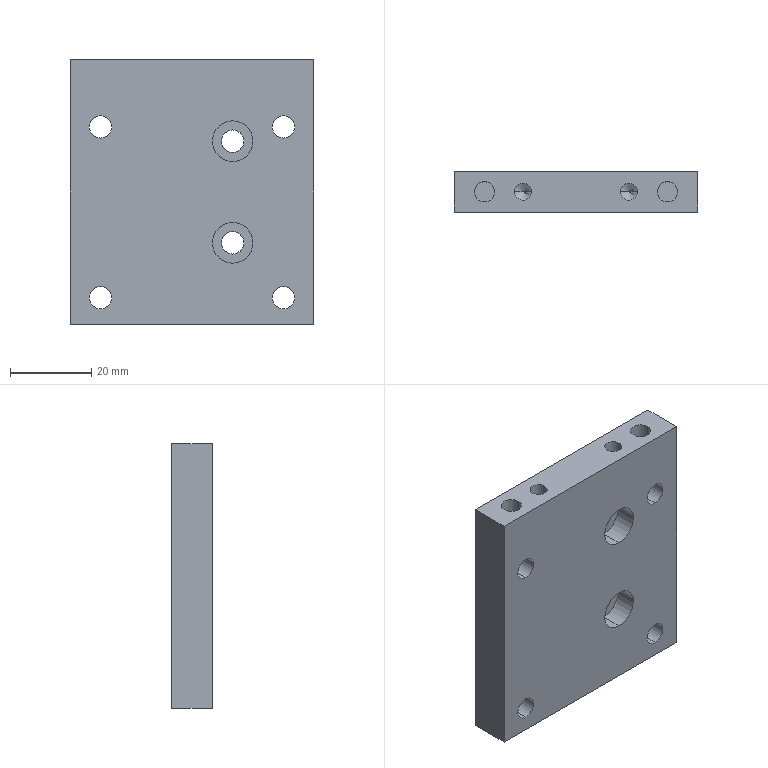Part | SolidWorks | features HoleWzd 4, Extrusion 1 | 1 solid | 50 faces | box 60 x 10 x 65 mm | volume 35169 mm3 | cylinder 32 | plane 14 | cone 4 | commonest cylinder face diameters 5.5 x12 10 x12 4.2 x4 5 x4
STEP:
#1=CARTESIAN_POINT('',(10.,0.4,17.5));
#2=VERTEX_POINT('',#1);
#3=CARTESIAN_POINT('',(10.,0.4,7.5));
#4=VERTEX_POINT('',#3);
#5=CARTESIAN_POINT('',(10.,0.4,12.5));
#6=DIRECTION('',(0.,-1.,0.));
#7=DIRECTION('',(0.,0.,-1.));
#8=AXIS2_PLACEMENT_3D('',#5,#6,#7);
#9=CIRCLE('',#8,5.);
#10=EDGE_CURVE('',#2,#4,#9,.T.);
#11=ORIENTED_EDGE('',*,*,#10,.F.);
#12=CARTESIAN_POINT('',(10.,-5.,17.5));
#13=VERTEX_POINT('',#12);
#14=CARTESIAN_POINT('',(10.,-5.,17.5));
#15=DIRECTION('',(0.,-1.,0.));
#16=VECTOR('',#15,1000.);
#17=LINE('',#14,#16);
#18=EDGE_CURVE('',#2,#13,#17,.T.);
#19=ORIENTED_EDGE('',*,*,#18,.T.);
#20=CARTESIAN_POINT('',(10.,-5.,7.5));
#21=VERTEX_POINT('',#20);
#22=CARTESIAN_POINT('',(10.,-5.,12.5));
#23=DIRECTION('',(0.,-1.,0.));
#24=DIRECTION('',(0.,0.,-1.));
#25=AXIS2_PLACEMENT_3D('',#22,#23,#24);
#26=CIRCLE('',#25,5.);
#27=EDGE_CURVE('',#13,#21,#26,.T.);
#28=ORIENTED_EDGE('',*,*,#27,.T.);
#29=CARTESIAN_POINT('',(10.,-5.,7.5));
#30=DIRECTION('',(0.,-1.,0.));
#31=VECTOR('',#30,1000.);
#32=LINE('',#29,#31);
#33=EDGE_CURVE('',#4,#21,#32,.T.);
#34=ORIENTED_EDGE('',*,*,#33,.F.);
#35=EDGE_LOOP('',(#11,#19,#28,#34));
#36=FACE_OUTER_BOUND('',#35,.T.);
#37=CARTESIAN_POINT('',(10.,-5.,12.5));
#38=DIRECTION('',(0.,-1.,0.));
#39=DIRECTION('',(0.,0.,-1.));
#40=AXIS2_PLACEMENT_3D('',#37,#38,#39);
#41=CYLINDRICAL_SURFACE('',#40,5.);
#42=ADVANCED_FACE('',(#36),#41,.F.);
#43=CARTESIAN_POINT('',(10.,5.,15.25));
#44=VERTEX_POINT('',#43);
#45=CARTESIAN_POINT('',(10.,5.,9.75));
#46=VERTEX_POINT('',#45);
#47=CARTESIAN_POINT('',(10.,5.,12.5));
#48=DIRECTION('',(0.,-1.,0.));
#49=DIRECTION('',(0.,0.,-1.));
#50=AXIS2_PLACEMENT_3D('',#47,#48,#49);
#51=CIRCLE('',#50,2.75);
#52=EDGE_CURVE('',#44,#46,#51,.T.);
#53=ORIENTED_EDGE('',*,*,#52,.F.);
#54=CARTESIAN_POINT('',(10.,0.4,15.25));
#55=VERTEX_POINT('',#54);
#56=CARTESIAN_POINT('',(10.,-5.,15.25));
#57=DIRECTION('',(0.,-1.,0.));
#58=VECTOR('',#57,1000.);
#59=LINE('',#56,#58);
#60=EDGE_CURVE('',#44,#55,#59,.T.);
#61=ORIENTED_EDGE('',*,*,#60,.T.);
#62=CARTESIAN_POINT('',(10.,0.4,9.75));
#63=VERTEX_POINT('',#62);
#64=CARTESIAN_POINT('',(10.,0.4,12.5));
#65=DIRECTION('',(0.,-1.,0.));
#66=DIRECTION('',(0.,0.,-1.));
#67=AXIS2_PLACEMENT_3D('',#64,#65,#66);
#68=CIRCLE('',#67,2.75);
#69=EDGE_CURVE('',#55,#63,#68,.T.);
#70=ORIENTED_EDGE('',*,*,#69,.T.);
#71=CARTESIAN_POINT('',(10.,-5.,9.75));
#72=DIRECTION('',(0.,-1.,0.));
#73=VECTOR('',#72,1000.);
#74=LINE('',#71,#73);
#75=EDGE_CURVE('',#46,#63,#74,.T.);
#76=ORIENTED_EDGE('',*,*,#75,.F.);
#77=EDGE_LOOP('',(#53,#61,#70,#76));
#78=FACE_OUTER_BOUND('',#77,.T.);
#79=CARTESIAN_POINT('',(10.,-5.,12.5));
#80=DIRECTION('',(0.,-1.,0.));
#81=DIRECTION('',(0.,0.,-1.));
#82=AXIS2_PLACEMENT_3D('',#79,#80,#81);
#83=CYLINDRICAL_SURFACE('',#82,2.75);
#84=ADVANCED_FACE('',(#78),#83,.F.);
#85=CARTESIAN_POINT('',(10.,0.4,-7.5));
#86=VERTEX_POINT('',#85);
#87=CARTESIAN_POINT('',(10.,0.4,-17.5));
#88=VERTEX_POINT('',#87);
#89=CARTESIAN_POINT('',(10.,0.4,-12.5));
#90=DIRECTION('',(0.,-1.,0.));
#91=DIRECTION('',(0.,0.,-1.));
#92=AXIS2_PLACEMENT_3D('',#89,#90,#91);
#93=CIRCLE('',#92,5.);
#94=EDGE_CURVE('',#86,#88,#93,.T.);
#95=ORIENTED_EDGE('',*,*,#94,.F.);
#96=CARTESIAN_POINT('',(10.,-5.,-7.5));
#97=VERTEX_POINT('',#96);
#98=CARTESIAN_POINT('',(10.,-5.,-7.5));
#99=DIRECTION('',(0.,-1.,0.));
#100=VECTOR('',#99,1000.);
#101=LINE('',#98,#100);
#102=EDGE_CURVE('',#86,#97,#101,.T.);
#103=ORIENTED_EDGE('',*,*,#102,.T.);
#104=CARTESIAN_POINT('',(10.,-5.,-17.5));
#105=VERTEX_POINT('',#104);
#106=CARTESIAN_POINT('',(10.,-5.,-12.5));
#107=DIRECTION('',(0.,-1.,0.));
#108=DIRECTION('',(0.,0.,-1.));
#109=AXIS2_PLACEMENT_3D('',#106,#107,#108);
#110=CIRCLE('',#109,5.);
#111=EDGE_CURVE('',#97,#105,#110,.T.);
#112=ORIENTED_EDGE('',*,*,#111,.T.);
#113=CARTESIAN_POINT('',(10.,-5.,-17.5));
#114=DIRECTION('',(0.,-1.,0.));
#115=VECTOR('',#114,1000.);
#116=LINE('',#113,#115);
#117=EDGE_CURVE('',#88,#105,#116,.T.);
#118=ORIENTED_EDGE('',*,*,#117,.F.);
#119=EDGE_LOOP('',(#95,#103,#112,#118));
#120=FACE_OUTER_BOUND('',#119,.T.);
#121=CARTESIAN_POINT('',(10.,-5.,-12.5));
#122=DIRECTION('',(0.,-1.,0.));
#123=DIRECTION('',(0.,0.,-1.));
#124=AXIS2_PLACEMENT_3D('',#121,#122,#123);
#125=CYLINDRICAL_SURFACE('',#124,5.);
#126=ADVANCED_FACE('',(#120),#125,.F.);
#127=CARTESIAN_POINT('',(10.,5.,-9.75));
#128=VERTEX_POINT('',#127);
#129=CARTESIAN_POINT('',(10.,5.,-15.25));
#130=VERTEX_POINT('',#129);
#131=CARTESIAN_POINT('',(10.,5.,-12.5));
#132=DIRECTION('',(0.,-1.,0.));
#133=DIRECTION('',(0.,0.,-1.));
#134=AXIS2_PLACEMENT_3D('',#131,#132,#133);
#135=CIRCLE('',#134,2.75);
#136=EDGE_CURVE('',#128,#130,#135,.T.);
#137=ORIENTED_EDGE('',*,*,#136,.F.);
#138=CARTESIAN_POINT('',(10.,0.4,-9.75));
#139=VERTEX_POINT('',#138);
#140=CARTESIAN_POINT('',(10.,-5.,-9.75));
#141=DIRECTION('',(0.,-1.,0.));
#142=VECTOR('',#141,1000.);
#143=LINE('',#140,#142);
#144=EDGE_CURVE('',#128,#139,#143,.T.);
#145=ORIENTED_EDGE('',*,*,#144,.T.);
#146=CARTESIAN_POINT('',(10.,0.4,-15.25));
#147=VERTEX_POINT('',#146);
#148=CARTESIAN_POINT('',(10.,0.4,-12.5));
#149=DIRECTION('',(0.,-1.,0.));
#150=DIRECTION('',(0.,0.,-1.));
#151=AXIS2_PLACEMENT_3D('',#148,#149,#150);
#152=CIRCLE('',#151,2.75);
#153=EDGE_CURVE('',#139,#147,#152,.T.);
#154=ORIENTED_EDGE('',*,*,#153,.T.);
#155=CARTESIAN_POINT('',(10.,-5.,-15.25));
#156=DIRECTION('',(0.,-1.,0.));
#157=VECTOR('',#156,1000.);
#158=LINE('',#155,#157);
#159=EDGE_CURVE('',#130,#147,#158,.T.);
#160=ORIENTED_EDGE('',*,*,#159,.F.);
#161=EDGE_LOOP('',(#137,#145,#154,#160));
#162=FACE_OUTER_BOUND('',#161,.T.);
#163=CARTESIAN_POINT('',(10.,-5.,-12.5));
#164=DIRECTION('',(0.,-1.,0.));
#165=DIRECTION('',(0.,0.,-1.));
#166=AXIS2_PLACEMENT_3D('',#163,#164,#165);
#167=CYLINDRICAL_SURFACE('',#166,2.75);
#168=ADVANCED_FACE('',(#162),#167,.F.);
#169=CARTESIAN_POINT('',(-15.1,0.,20.1));
#170=VERTEX_POINT('',#169);
#171=CARTESIAN_POINT('',(-10.9,0.,20.1));
#172=VERTEX_POINT('',#171);
#173=CARTESIAN_POINT('',(-13.,0.,20.1));
#174=DIRECTION('',(0.,0.,1.));
#175=DIRECTION('',(1.,0.,0.));
#176=AXIS2_PLACEMENT_3D('',#173,#174,#175);
#177=CIRCLE('',#176,2.1);
#178=EDGE_CURVE('',#170,#172,#177,.T.);
#179=ORIENTED_EDGE('',*,*,#178,.F.);
#180=CARTESIAN_POINT('',(-15.1,0.,32.5));
#181=VERTEX_POINT('',#180);
#182=CARTESIAN_POINT('',(-15.1,0.,32.5));
#183=DIRECTION('',(0.,0.,1.));
#184=VECTOR('',#183,1000.);
#185=LINE('',#182,#184);
#186=EDGE_CURVE('',#170,#181,#185,.T.);
#187=ORIENTED_EDGE('',*,*,#186,.T.);
#188=CARTESIAN_POINT('',(-10.9,0.,32.5));
#189=VERTEX_POINT('',#188);
#190=CARTESIAN_POINT('',(-13.,0.,32.5));
#191=DIRECTION('',(0.,0.,1.));
#192=DIRECTION('',(1.,0.,0.));
#193=AXIS2_PLACEMENT_3D('',#190,#191,#192);
#194=CIRCLE('',#193,2.1);
#195=EDGE_CURVE('',#181,#189,#194,.T.);
#196=ORIENTED_EDGE('',*,*,#195,.T.);
#197=CARTESIAN_POINT('',(-10.9,0.,32.5));
#198=DIRECTION('',(0.,0.,1.));
#199=VECTOR('',#198,1000.);
#200=LINE('',#197,#199);
#201=EDGE_CURVE('',#172,#189,#200,.T.);
#202=ORIENTED_EDGE('',*,*,#201,.F.);
#203=EDGE_LOOP('',(#179,#187,#196,#202));
#204=FACE_OUTER_BOUND('',#203,.T.);
#205=CARTESIAN_POINT('',(-13.,0.,32.5));
#206=DIRECTION('',(0.,0.,1.));
#207=DIRECTION('',(1.,0.,0.));
#208=AXIS2_PLACEMENT_3D('',#205,#206,#207);
#209=CYLINDRICAL_SURFACE('',#208,2.1);
#210=ADVANCED_FACE('',(#204),#209,.F.);
#211=CARTESIAN_POINT('',(-13.,0.,18.838));
#212=VERTEX_POINT('',#211);
#213=CARTESIAN_POINT('',(-10.9,0.,20.1));
#214=DIRECTION('',(0.8572,0.,0.515));
#215=VECTOR('',#214,1000.);
#216=LINE('',#213,#215);
#217=EDGE_CURVE('',#212,#172,#216,.T.);
#218=ORIENTED_EDGE('',*,*,#217,.F.);
#219=CARTESIAN_POINT('',(-15.1,0.,20.1));
#220=DIRECTION('',(-0.8572,0.,0.515));
#221=VECTOR('',#220,1000.);
#222=LINE('',#219,#221);
#223=EDGE_CURVE('',#212,#170,#222,.T.);
#224=ORIENTED_EDGE('',*,*,#223,.T.);
#225=ORIENTED_EDGE('',*,*,#178,.T.);
#226=EDGE_LOOP('',(#218,#224,#225));
#227=FACE_OUTER_BOUND('',#226,.T.);
#228=CARTESIAN_POINT('',(-13.,0.,20.1));
#229=DIRECTION('',(0.,0.,1.));
#230=DIRECTION('',(1.,0.,0.));
#231=AXIS2_PLACEMENT_3D('',#228,#229,#230);
#232=CONICAL_SURFACE('',#231,2.1,1.03);
#233=ADVANCED_FACE('',(#227),#232,.F.);
#234=CARTESIAN_POINT('',(10.9,0.,20.1));
#235=VERTEX_POINT('',#234);
#236=CARTESIAN_POINT('',(15.1,0.,20.1));
#237=VERTEX_POINT('',#236);
#238=CARTESIAN_POINT('',(13.,0.,20.1));
#239=DIRECTION('',(0.,0.,1.));
#240=DIRECTION('',(1.,0.,0.));
#241=AXIS2_PLACEMENT_3D('',#238,#239,#240);
#242=CIRCLE('',#241,2.1);
#243=EDGE_CURVE('',#235,#237,#242,.T.);
#244=ORIENTED_EDGE('',*,*,#243,.F.);
#245=CARTESIAN_POINT('',(10.9,0.,32.5));
#246=VERTEX_POINT('',#245);
#247=CARTESIAN_POINT('',(10.9,0.,32.5));
#248=DIRECTION('',(0.,0.,1.));
#249=VECTOR('',#248,1000.);
#250=LINE('',#247,#249);
#251=EDGE_CURVE('',#235,#246,#250,.T.);
#252=ORIENTED_EDGE('',*,*,#251,.T.);
#253=CARTESIAN_POINT('',(15.1,0.,32.5));
#254=VERTEX_POINT('',#253);
#255=CARTESIAN_POINT('',(13.,0.,32.5));
#256=DIRECTION('',(0.,0.,1.));
#257=DIRECTION('',(1.,0.,0.));
#258=AXIS2_PLACEMENT_3D('',#255,#256,#257);
#259=CIRCLE('',#258,2.1);
#260=EDGE_CURVE('',#246,#254,#259,.T.);
#261=ORIENTED_EDGE('',*,*,#260,.T.);
#262=CARTESIAN_POINT('',(15.1,0.,32.5));
#263=DIRECTION('',(0.,0.,1.));
#264=VECTOR('',#263,1000.);
#265=LINE('',#262,#264);
#266=EDGE_CURVE('',#237,#254,#265,.T.);
#267=ORIENTED_EDGE('',*,*,#266,.F.);
#268=EDGE_LOOP('',(#244,#252,#261,#267));
#269=FACE_OUTER_BOUND('',#268,.T.);
#270=CARTESIAN_POINT('',(13.,0.,32.5));
#271=DIRECTION('',(0.,0.,1.));
#272=DIRECTION('',(1.,0.,0.));
#273=AXIS2_PLACEMENT_3D('',#270,#271,#272);
#274=CYLINDRICAL_SURFACE('',#273,2.1);
#275=ADVANCED_FACE('',(#269),#274,.F.);
#276=CARTESIAN_POINT('',(13.,0.,18.838));
#277=VERTEX_POINT('',#276);
#278=CARTESIAN_POINT('',(15.1,0.,20.1));
#279=DIRECTION('',(0.8572,0.,0.515));
#280=VECTOR('',#279,1000.);
#281=LINE('',#278,#280);
#282=EDGE_CURVE('',#277,#237,#281,.T.);
#283=ORIENTED_EDGE('',*,*,#282,.F.);
#284=CARTESIAN_POINT('',(10.9,0.,20.1));
#285=DIRECTION('',(-0.8572,0.,0.515));
#286=VECTOR('',#285,1000.);
#287=LINE('',#284,#286);
#288=EDGE_CURVE('',#277,#235,#287,.T.);
#289=ORIENTED_EDGE('',*,*,#288,.T.);
#290=ORIENTED_EDGE('',*,*,#243,.T.);
#291=EDGE_LOOP('',(#283,#289,#290));
#292=FACE_OUTER_BOUND('',#291,.T.);
#293=CARTESIAN_POINT('',(13.,0.,20.1));
#294=DIRECTION('',(0.,0.,1.));
#295=DIRECTION('',(1.,0.,0.));
#296=AXIS2_PLACEMENT_3D('',#293,#294,#295);
#297=CONICAL_SURFACE('',#296,2.1,1.03);
#298=ADVANCED_FACE('',(#292),#297,.F.);
#299=CARTESIAN_POINT('',(-25.,0.,25.5));
#300=VERTEX_POINT('',#299);
#301=CARTESIAN_POINT('',(-20.,0.,25.5));
#302=VERTEX_POINT('',#301);
#303=CARTESIAN_POINT('',(-22.5,0.,25.5));
#304=DIRECTION('',(0.,0.,1.));
#305=DIRECTION('',(1.,0.,0.));
#306=AXIS2_PLACEMENT_3D('',#303,#304,#305);
#307=CIRCLE('',#306,2.5);
#308=EDGE_CURVE('',#300,#302,#307,.T.);
#309=ORIENTED_EDGE('',*,*,#308,.F.);
#310=CARTESIAN_POINT('',(-25.,0.,32.5));
#311=VERTEX_POINT('',#310);
#312=CARTESIAN_POINT('',(-25.,0.,32.5));
#313=DIRECTION('',(0.,0.,1.));
#314=VECTOR('',#313,1000.);
#315=LINE('',#312,#314);
#316=EDGE_CURVE('',#300,#311,#315,.T.);
#317=ORIENTED_EDGE('',*,*,#316,.T.);
#318=CARTESIAN_POINT('',(-20.,0.,32.5));
#319=VERTEX_POINT('',#318);
#320=CARTESIAN_POINT('',(-22.5,0.,32.5));
#321=DIRECTION('',(0.,0.,1.));
#322=DIRECTION('',(1.,0.,0.));
#323=AXIS2_PLACEMENT_3D('',#320,#321,#322);
#324=CIRCLE('',#323,2.5);
#325=EDGE_CURVE('',#311,#319,#324,.T.);
#326=ORIENTED_EDGE('',*,*,#325,.T.);
#327=CARTESIAN_POINT('',(-20.,0.,32.5));
#328=DIRECTION('',(0.,0.,1.));
#329=VECTOR('',#328,1000.);
#330=LINE('',#327,#329);
#331=EDGE_CURVE('',#302,#319,#330,.T.);
#332=ORIENTED_EDGE('',*,*,#331,.F.);
#333=EDGE_LOOP('',(#309,#317,#326,#332));
#334=FACE_OUTER_BOUND('',#333,.T.);
#335=CARTESIAN_POINT('',(-22.5,0.,32.5));
#336=DIRECTION('',(0.,0.,1.));
#337=DIRECTION('',(1.,0.,0.));
#338=AXIS2_PLACEMENT_3D('',#335,#336,#337);
#339=CYLINDRICAL_SURFACE('',#338,2.5);
#340=ADVANCED_FACE('',(#334),#339,.F.);
#341=CARTESIAN_POINT('',(20.,0.,25.5));
#342=VERTEX_POINT('',#341);
#343=CARTESIAN_POINT('',(25.,0.,25.5));
#344=VERTEX_POINT('',#343);
#345=CARTESIAN_POINT('',(22.5,0.,25.5));
#346=DIRECTION('',(0.,0.,1.));
#347=DIRECTION('',(1.,0.,0.));
#348=AXIS2_PLACEMENT_3D('',#345,#346,#347);
#349=CIRCLE('',#348,2.5);
#350=EDGE_CURVE('',#342,#344,#349,.T.);
#351=ORIENTED_EDGE('',*,*,#350,.F.);
#352=CARTESIAN_POINT('',(20.,0.,32.5));
#353=VERTEX_POINT('',#352);
#354=CARTESIAN_POINT('',(20.,0.,32.5));
#355=DIRECTION('',(0.,0.,1.));
#356=VECTOR('',#355,1000.);
#357=LINE('',#354,#356);
#358=EDGE_CURVE('',#342,#353,#357,.T.);
#359=ORIENTED_EDGE('',*,*,#358,.T.);
#360=CARTESIAN_POINT('',(25.,0.,32.5));
#361=VERTEX_POINT('',#360);
#362=CARTESIAN_POINT('',(22.5,0.,32.5));
#363=DIRECTION('',(0.,0.,1.));
#364=DIRECTION('',(1.,0.,0.));
#365=AXIS2_PLACEMENT_3D('',#362,#363,#364);
#366=CIRCLE('',#365,2.5);
#367=EDGE_CURVE('',#353,#361,#366,.T.);
#368=ORIENTED_EDGE('',*,*,#367,.T.);
#369=CARTESIAN_POINT('',(25.,0.,32.5));
#370=DIRECTION('',(0.,0.,1.));
#371=VECTOR('',#370,1000.);
#372=LINE('',#369,#371);
#373=EDGE_CURVE('',#344,#361,#372,.T.);
#374=ORIENTED_EDGE('',*,*,#373,.F.);
#375=EDGE_LOOP('',(#351,#359,#368,#374));
#376=FACE_OUTER_BOUND('',#375,.T.);
#377=CARTESIAN_POINT('',(22.5,0.,32.5));
#378=DIRECTION('',(0.,0.,1.));
#379=DIRECTION('',(1.,0.,0.));
#380=AXIS2_PLACEMENT_3D('',#377,#378,#379);
#381=CYLINDRICAL_SURFACE('',#380,2.5);
#382=ADVANCED_FACE('',(#376),#381,.F.);
#383=CARTESIAN_POINT('',(-22.5,-0.4,-31.));
#384=VERTEX_POINT('',#383);
#385=CARTESIAN_POINT('',(-22.5,-0.4,-21.));
#386=VERTEX_POINT('',#385);
#387=CARTESIAN_POINT('',(-22.5,-0.4,-26.));
#388=DIRECTION('',(0.,1.,0.));
#389=DIRECTION('',(0.,0.,1.));
#390=AXIS2_PLACEMENT_3D('',#387,#388,#389);
#391=CIRCLE('',#390,5.);
#392=EDGE_CURVE('',#384,#386,#391,.T.);
#393=ORIENTED_EDGE('',*,*,#392,.F.);
#394=CARTESIAN_POINT('',(-22.5,5.,-31.));
#395=VERTEX_POINT('',#394);
#396=CARTESIAN_POINT('',(-22.5,5.,-31.));
#397=DIRECTION('',(0.,1.,0.));
#398=VECTOR('',#397,1000.);
#399=LINE('',#396,#398);
#400=EDGE_CURVE('',#384,#395,#399,.T.);
#401=ORIENTED_EDGE('',*,*,#400,.T.);
#402=CARTESIAN_POINT('',(-22.5,5.,-21.));
#403=VERTEX_POINT('',#402);
#404=CARTESIAN_POINT('',(-22.5,5.,-26.));
#405=DIRECTION('',(0.,1.,0.));
#406=DIRECTION('',(0.,0.,1.));
#407=AXIS2_PLACEMENT_3D('',#404,#405,#406);
#408=CIRCLE('',#407,5.);
#409=EDGE_CURVE('',#395,#403,#408,.T.);
#410=ORIENTED_EDGE('',*,*,#409,.T.);
#411=CARTESIAN_POINT('',(-22.5,5.,-21.));
#412=DIRECTION('',(0.,1.,0.));
#413=VECTOR('',#412,1000.);
#414=LINE('',#411,#413);
#415=EDGE_CURVE('',#386,#403,#414,.T.);
#416=ORIENTED_EDGE('',*,*,#415,.F.);
#417=EDGE_LOOP('',(#393,#401,#410,#416));
#418=FACE_OUTER_BOUND('',#417,.T.);
#419=CARTESIAN_POINT('',(-22.5,5.,-26.));
#420=DIRECTION('',(0.,1.,0.));
#421=DIRECTION('',(0.,0.,1.));
#422=AXIS2_PLACEMENT_3D('',#419,#420,#421);
#423=CYLINDRICAL_SURFACE('',#422,5.);
#424=ADVANCED_FACE('',(#418),#423,.F.);
#425=CARTESIAN_POINT('',(-22.5,-5.,-28.75));
#426=VERTEX_POINT('',#425);
#427=CARTESIAN_POINT('',(-22.5,-5.,-23.25));
#428=VERTEX_POINT('',#427);
#429=CARTESIAN_POINT('',(-22.5,-5.,-26.));
#430=DIRECTION('',(0.,1.,0.));
#431=DIRECTION('',(0.,0.,1.));
#432=AXIS2_PLACEMENT_3D('',#429,#430,#431);
#433=CIRCLE('',#432,2.75);
#434=EDGE_CURVE('',#426,#428,#433,.T.);
#435=ORIENTED_EDGE('',*,*,#434,.F.);
#436=CARTESIAN_POINT('',(-22.5,-0.4,-28.75));
#437=VERTEX_POINT('',#436);
#438=CARTESIAN_POINT('',(-22.5,5.,-28.75));
#439=DIRECTION('',(0.,1.,0.));
#440=VECTOR('',#439,1000.);
#441=LINE('',#438,#440);
#442=EDGE_CURVE('',#426,#437,#441,.T.);
#443=ORIENTED_EDGE('',*,*,#442,.T.);
#444=CARTESIAN_POINT('',(-22.5,-0.4,-23.25));
#445=VERTEX_POINT('',#444);
#446=CARTESIAN_POINT('',(-22.5,-0.4,-26.));
#447=DIRECTION('',(0.,1.,0.));
#448=DIRECTION('',(0.,0.,1.));
#449=AXIS2_PLACEMENT_3D('',#446,#447,#448);
#450=CIRCLE('',#449,2.75);
#451=EDGE_CURVE('',#437,#445,#450,.T.);
#452=ORIENTED_EDGE('',*,*,#451,.T.);
#453=CARTESIAN_POINT('',(-22.5,5.,-23.25));
#454=DIRECTION('',(0.,1.,0.));
#455=VECTOR('',#454,1000.);
#456=LINE('',#453,#455);
#457=EDGE_CURVE('',#428,#445,#456,.T.);
#458=ORIENTED_EDGE('',*,*,#457,.F.);
#459=EDGE_LOOP('',(#435,#443,#452,#458));
#460=FACE_OUTER_BOUND('',#459,.T.);
#461=CARTESIAN_POINT('',(-22.5,5.,-26.));
#462=DIRECTION('',(0.,1.,0.));
#463=DIRECTION('',(0.,0.,1.));
#464=AXIS2_PLACEMENT_3D('',#461,#462,#463);
#465=CYLINDRICAL_SURFACE('',#464,2.75);
#466=ADVANCED_FACE('',(#460),#465,.F.);
#467=CARTESIAN_POINT('',(-22.5,-0.4,11.));
#468=VERTEX_POINT('',#467);
#469=CARTESIAN_POINT('',(-22.5,-0.4,21.));
#470=VERTEX_POINT('',#469);
#471=CARTESIAN_POINT('',(-22.5,-0.4,16.));
#472=DIRECTION('',(0.,1.,0.));
#473=DIRECTION('',(0.,0.,1.));
#474=AXIS2_PLACEMENT_3D('',#471,#472,#473);
#475=CIRCLE('',#474,5.);
#476=EDGE_CURVE('',#468,#470,#475,.T.);
#477=ORIENTED_EDGE('',*,*,#476,.F.);
#478=CARTESIAN_POINT('',(-22.5,5.,11.));
#479=VERTEX_POINT('',#478);
#480=CARTESIAN_POINT('',(-22.5,5.,11.));
#481=DIRECTION('',(0.,1.,0.));
#482=VECTOR('',#481,1000.);
#483=LINE('',#480,#482);
#484=EDGE_CURVE('',#468,#479,#483,.T.);
#485=ORIENTED_EDGE('',*,*,#484,.T.);
#486=CARTESIAN_POINT('',(-22.5,5.,21.));
#487=VERTEX_POINT('',#486);
#488=CARTESIAN_POINT('',(-22.5,5.,16.));
#489=DIRECTION('',(0.,1.,0.));
#490=DIRECTION('',(0.,0.,1.));
#491=AXIS2_PLACEMENT_3D('',#488,#489,#490);
#492=CIRCLE('',#491,5.);
#493=EDGE_CURVE('',#479,#487,#492,.T.);
#494=ORIENTED_EDGE('',*,*,#493,.T.);
#495=CARTESIAN_POINT('',(-22.5,5.,21.));
#496=DIRECTION('',(0.,1.,0.));
#497=VECTOR('',#496,1000.);
#498=LINE('',#495,#497);
#499=EDGE_CURVE('',#470,#487,#498,.T.);
#500=ORIENTED_EDGE('',*,*,#499,.F.);
#501=EDGE_LOOP('',(#477,#485,#494,#500));
#502=FACE_OUTER_BOUND('',#501,.T.);
#503=CARTESIAN_POINT('',(-22.5,5.,16.));
#504=DIRECTION('',(0.,1.,0.));
#505=DIRECTION('',(0.,0.,1.));
#506=AXIS2_PLACEMENT_3D('',#503,#504,#505);
#507=CYLINDRICAL_SURFACE('',#506,5.);
#508=ADVANCED_FACE('',(#502),#507,.F.);
#509=CARTESIAN_POINT('',(-22.5,-5.,13.25));
#510=VERTEX_POINT('',#509);
#511=CARTESIAN_POINT('',(-22.5,-5.,18.75));
#512=VERTEX_POINT('',#511);
#513=CARTESIAN_POINT('',(-22.5,-5.,16.));
#514=DIRECTION('',(0.,1.,0.));
#515=DIRECTION('',(0.,0.,1.));
#516=AXIS2_PLACEMENT_3D('',#513,#514,#515);
#517=CIRCLE('',#516,2.75);
#518=EDGE_CURVE('',#510,#512,#517,.T.);
#519=ORIENTED_EDGE('',*,*,#518,.F.);
#520=CARTESIAN_POINT('',(-22.5,-0.4,13.25));
#521=VERTEX_POINT('',#520);
#522=CARTESIAN_POINT('',(-22.5,5.,13.25));
#523=DIRECTION('',(0.,1.,0.));
#524=VECTOR('',#523,1000.);
#525=LINE('',#522,#524);
#526=EDGE_CURVE('',#510,#521,#525,.T.);
#527=ORIENTED_EDGE('',*,*,#526,.T.);
#528=CARTESIAN_POINT('',(-22.5,-0.4,18.75));
#529=VERTEX_POINT('',#528);
#530=CARTESIAN_POINT('',(-22.5,-0.4,16.));
#531=DIRECTION('',(0.,1.,0.));
#532=DIRECTION('',(0.,0.,1.));
#533=AXIS2_PLACEMENT_3D('',#530,#531,#532);
#534=CIRCLE('',#533,2.75);
#535=EDGE_CURVE('',#521,#529,#534,.T.);
#536=ORIENTED_EDGE('',*,*,#535,.T.);
#537=CARTESIAN_POINT('',(-22.5,5.,18.75));
#538=DIRECTION('',(0.,1.,0.));
#539=VECTOR('',#538,1000.);
#540=LINE('',#537,#539);
#541=EDGE_CURVE('',#512,#529,#540,.T.);
#542=ORIENTED_EDGE('',*,*,#541,.F.);
#543=EDGE_LOOP('',(#519,#527,#536,#542));
#544=FACE_OUTER_BOUND('',#543,.T.);
#545=CARTESIAN_POINT('',(-22.5,5.,16.));
#546=DIRECTION('',(0.,1.,0.));
#547=DIRECTION('',(0.,0.,1.));
#548=AXIS2_PLACEMENT_3D('',#545,#546,#547);
#549=CYLINDRICAL_SURFACE('',#548,2.75);
#550=ADVANCED_FACE('',(#544),#549,.F.);
#551=CARTESIAN_POINT('',(22.5,-0.4,11.));
#552=VERTEX_POINT('',#551);
#553=CARTESIAN_POINT('',(22.5,-0.4,21.));
#554=VERTEX_POINT('',#553);
#555=CARTESIAN_POINT('',(22.5,-0.4,16.));
#556=DIRECTION('',(0.,1.,0.));
#557=DIRECTION('',(0.,0.,1.));
#558=AXIS2_PLACEMENT_3D('',#555,#556,#557);
#559=CIRCLE('',#558,5.);
#560=EDGE_CURVE('',#552,#554,#559,.T.);
#561=ORIENTED_EDGE('',*,*,#560,.F.);
#562=CARTESIAN_POINT('',(22.5,5.,11.));
#563=VERTEX_POINT('',#562);
#564=CARTESIAN_POINT('',(22.5,5.,11.));
#565=DIRECTION('',(0.,1.,0.));
#566=VECTOR('',#565,1000.);
#567=LINE('',#564,#566);
#568=EDGE_CURVE('',#552,#563,#567,.T.);
#569=ORIENTED_EDGE('',*,*,#568,.T.);
#570=CARTESIAN_POINT('',(22.5,5.,21.));
#571=VERTEX_POINT('',#570);
#572=CARTESIAN_POINT('',(22.5,5.,16.));
#573=DIRECTION('',(0.,1.,0.));
#574=DIRECTION('',(0.,0.,1.));
#575=AXIS2_PLACEMENT_3D('',#572,#573,#574);
#576=CIRCLE('',#575,5.);
#577=EDGE_CURVE('',#563,#571,#576,.T.);
#578=ORIENTED_EDGE('',*,*,#577,.T.);
#579=CARTESIAN_POINT('',(22.5,5.,21.));
#580=DIRECTION('',(0.,1.,0.));
#581=VECTOR('',#580,1000.);
#582=LINE('',#579,#581);
#583=EDGE_CURVE('',#554,#571,#582,.T.);
#584=ORIENTED_EDGE('',*,*,#583,.F.);
#585=EDGE_LOOP('',(#561,#569,#578,#584));
#586=FACE_OUTER_BOUND('',#585,.T.);
#587=CARTESIAN_POINT('',(22.5,5.,16.));
#588=DIRECTION('',(0.,1.,0.));
#589=DIRECTION('',(0.,0.,1.));
#590=AXIS2_PLACEMENT_3D('',#587,#588,#589);
#591=CYLINDRICAL_SURFACE('',#590,5.);
#592=ADVANCED_FACE('',(#586),#591,.F.);
#593=CARTESIAN_POINT('',(22.5,-5.,13.25));
#594=VERTEX_POINT('',#593);
#595=CARTESIAN_POINT('',(22.5,-5.,18.75));
#596=VERTEX_POINT('',#595);
#597=CARTESIAN_POINT('',(22.5,-5.,16.));
#598=DIRECTION('',(0.,1.,0.));
#599=DIRECTION('',(0.,0.,1.));
#600=AXIS2_PLACEMENT_3D('',#597,#598,#599);
#601=CIRCLE('',#600,2.75);
#602=EDGE_CURVE('',#594,#596,#601,.T.);
#603=ORIENTED_EDGE('',*,*,#602,.F.);
#604=CARTESIAN_POINT('',(22.5,-0.4,13.25));
#605=VERTEX_POINT('',#604);
#606=CARTESIAN_POINT('',(22.5,5.,13.25));
#607=DIRECTION('',(0.,1.,0.));
#608=VECTOR('',#607,1000.);
#609=LINE('',#606,#608);
#610=EDGE_CURVE('',#594,#605,#609,.T.);
#611=ORIENTED_EDGE('',*,*,#610,.T.);
#612=CARTESIAN_POINT('',(22.5,-0.4,18.75));
#613=VERTEX_POINT('',#612);
#614=CARTESIAN_POINT('',(22.5,-0.4,16.));
#615=DIRECTION('',(0.,1.,0.));
#616=DIRECTION('',(0.,0.,1.));
#617=AXIS2_PLACEMENT_3D('',#614,#615,#616);
#618=CIRCLE('',#617,2.75);
#619=EDGE_CURVE('',#605,#613,#618,.T.);
#620=ORIENTED_EDGE('',*,*,#619,.T.);
#621=CARTESIAN_POINT('',(22.5,5.,18.75));
#622=DIRECTION('',(0.,1.,0.));
#623=VECTOR('',#622,1000.);
#624=LINE('',#621,#623);
#625=EDGE_CURVE('',#596,#613,#624,.T.);
#626=ORIENTED_EDGE('',*,*,#625,.F.);
#627=EDGE_LOOP('',(#603,#611,#620,#626));
#628=FACE_OUTER_BOUND('',#627,.T.);
#629=CARTESIAN_POINT('',(22.5,5.,16.));
#630=DIRECTION('',(0.,1.,0.));
#631=DIRECTION('',(0.,0.,1.));
#632=AXIS2_PLACEMENT_3D('',#629,#630,#631);
#633=CYLINDRICAL_SURFACE('',#632,2.75);
#634=ADVANCED_FACE('',(#628),#633,.F.);
#635=CARTESIAN_POINT('',(22.5,-0.4,-31.));
#636=VERTEX_POINT('',#635);
#637=CARTESIAN_POINT('',(22.5,-0.4,-21.));
#638=VERTEX_POINT('',#637);
#639=CARTESIAN_POINT('',(22.5,-0.4,-26.));
#640=DIRECTION('',(0.,1.,0.));
#641=DIRECTION('',(0.,0.,1.));
#642=AXIS2_PLACEMENT_3D('',#639,#640,#641);
#643=CIRCLE('',#642,5.);
#644=EDGE_CURVE('',#636,#638,#643,.T.);
#645=ORIENTED_EDGE('',*,*,#644,.F.);
#646=CARTESIAN_POINT('',(22.5,5.,-31.));
#647=VERTEX_POINT('',#646);
#648=CARTESIAN_POINT('',(22.5,5.,-31.));
#649=DIRECTION('',(0.,1.,0.));
#650=VECTOR('',#649,1000.);
#651=LINE('',#648,#650);
#652=EDGE_CURVE('',#636,#647,#651,.T.);
#653=ORIENTED_EDGE('',*,*,#652,.T.);
#654=CARTESIAN_POINT('',(22.5,5.,-21.));
#655=VERTEX_POINT('',#654);
#656=CARTESIAN_POINT('',(22.5,5.,-26.));
#657=DIRECTION('',(0.,1.,0.));
#658=DIRECTION('',(0.,0.,1.));
#659=AXIS2_PLACEMENT_3D('',#656,#657,#658);
#660=CIRCLE('',#659,5.);
#661=EDGE_CURVE('',#647,#655,#660,.T.);
#662=ORIENTED_EDGE('',*,*,#661,.T.);
#663=CARTESIAN_POINT('',(22.5,5.,-21.));
#664=DIRECTION('',(0.,1.,0.));
#665=VECTOR('',#664,1000.);
#666=LINE('',#663,#665);
#667=EDGE_CURVE('',#638,#655,#666,.T.);
#668=ORIENTED_EDGE('',*,*,#667,.F.);
#669=EDGE_LOOP('',(#645,#653,#662,#668));
#670=FACE_OUTER_BOUND('',#669,.T.);
#671=CARTESIAN_POINT('',(22.5,5.,-26.));
#672=DIRECTION('',(0.,1.,0.));
#673=DIRECTION('',(0.,0.,1.));
#674=AXIS2_PLACEMENT_3D('',#671,#672,#673);
#675=CYLINDRICAL_SURFACE('',#674,5.);
#676=ADVANCED_FACE('',(#670),#675,.F.);
#677=CARTESIAN_POINT('',(22.5,-5.,-28.75));
#678=VERTEX_POINT('',#677);
#679=CARTESIAN_POINT('',(22.5,-5.,-23.25));
#680=VERTEX_POINT('',#679);
#681=CARTESIAN_POINT('',(22.5,-5.,-26.));
#682=DIRECTION('',(0.,1.,0.));
#683=DIRECTION('',(0.,0.,1.));
#684=AXIS2_PLACEMENT_3D('',#681,#682,#683);
#685=CIRCLE('',#684,2.75);
#686=EDGE_CURVE('',#678,#680,#685,.T.);
#687=ORIENTED_EDGE('',*,*,#686,.F.);
#688=CARTESIAN_POINT('',(22.5,-0.4,-28.75));
#689=VERTEX_POINT('',#688);
#690=CARTESIAN_POINT('',(22.5,5.,-28.75));
#691=DIRECTION('',(0.,1.,0.));
#692=VECTOR('',#691,1000.);
#693=LINE('',#690,#692);
#694=EDGE_CURVE('',#678,#689,#693,.T.);
#695=ORIENTED_EDGE('',*,*,#694,.T.);
#696=CARTESIAN_POINT('',(22.5,-0.4,-23.25));
#697=VERTEX_POINT('',#696);
#698=CARTESIAN_POINT('',(22.5,-0.4,-26.));
#699=DIRECTION('',(0.,1.,0.));
#700=DIRECTION('',(0.,0.,1.));
#701=AXIS2_PLACEMENT_3D('',#698,#699,#700);
#702=CIRCLE('',#701,2.75);
#703=EDGE_CURVE('',#689,#697,#702,.T.);
#704=ORIENTED_EDGE('',*,*,#703,.T.);
#705=CARTESIAN_POINT('',(22.5,5.,-23.25));
#706=DIRECTION('',(0.,1.,0.));
#707=VECTOR('',#706,1000.);
#708=LINE('',#705,#707);
#709=EDGE_CURVE('',#680,#697,#708,.T.);
#710=ORIENTED_EDGE('',*,*,#709,.F.);
#711=EDGE_LOOP('',(#687,#695,#704,#710));
#712=FACE_OUTER_BOUND('',#711,.T.);
#713=CARTESIAN_POINT('',(22.5,5.,-26.));
#714=DIRECTION('',(0.,1.,0.));
#715=DIRECTION('',(0.,0.,1.));
#716=AXIS2_PLACEMENT_3D('',#713,#714,#715);
#717=CYLINDRICAL_SURFACE('',#716,2.75);
#718=ADVANCED_FACE('',(#712),#717,.F.);
#719=CARTESIAN_POINT('',(10.,-5.,12.5));
#720=DIRECTION('',(0.,-1.,0.));
#721=DIRECTION('',(0.,0.,-1.));
#722=AXIS2_PLACEMENT_3D('',#719,#720,#721);
#723=CIRCLE('',#722,5.);
#724=EDGE_CURVE('',#21,#13,#723,.T.);
#725=ORIENTED_EDGE('',*,*,#724,.F.);
#726=ORIENTED_EDGE('',*,*,#27,.F.);
#727=EDGE_LOOP('',(#725,#726));
#728=FACE_BOUND('',#727,.T.);
#729=CARTESIAN_POINT('',(-22.5,-5.,-26.));
#730=DIRECTION('',(0.,1.,0.));
#731=DIRECTION('',(0.,0.,1.));
#732=AXIS2_PLACEMENT_3D('',#729,#730,#731);
#733=CIRCLE('',#732,2.75);
#734=EDGE_CURVE('',#428,#426,#733,.T.);
#735=ORIENTED_EDGE('',*,*,#734,.T.);
#736=ORIENTED_EDGE('',*,*,#434,.T.);
#737=EDGE_LOOP('',(#735,#736));
#738=FACE_BOUND('',#737,.T.);
#739=CARTESIAN_POINT('',(-22.5,-5.,16.));
#740=DIRECTION('',(0.,1.,0.));
#741=DIRECTION('',(0.,0.,1.));
#742=AXIS2_PLACEMENT_3D('',#739,#740,#741);
#743=CIRCLE('',#742,2.75);
#744=EDGE_CURVE('',#512,#510,#743,.T.);
#745=ORIENTED_EDGE('',*,*,#744,.T.);
#746=ORIENTED_EDGE('',*,*,#518,.T.);
#747=EDGE_LOOP('',(#745,#746));
#748=FACE_BOUND('',#747,.T.);
#749=CARTESIAN_POINT('',(22.5,-5.,16.));
#750=DIRECTION('',(0.,1.,0.));
#751=DIRECTION('',(0.,0.,1.));
#752=AXIS2_PLACEMENT_3D('',#749,#750,#751);
#753=CIRCLE('',#752,2.75);
#754=EDGE_CURVE('',#596,#594,#753,.T.);
#755=ORIENTED_EDGE('',*,*,#754,.T.);
#756=ORIENTED_EDGE('',*,*,#602,.T.);
#757=EDGE_LOOP('',(#755,#756));
#758=FACE_BOUND('',#757,.T.);
#759=CARTESIAN_POINT('',(22.5,-5.,-26.));
#760=DIRECTION('',(0.,1.,0.));
#761=DIRECTION('',(0.,0.,1.));
#762=AXIS2_PLACEMENT_3D('',#759,#760,#761);
#763=CIRCLE('',#762,2.75);
#764=EDGE_CURVE('',#680,#678,#763,.T.);
#765=ORIENTED_EDGE('',*,*,#764,.T.);
#766=ORIENTED_EDGE('',*,*,#686,.T.);
#767=EDGE_LOOP('',(#765,#766));
#768=FACE_BOUND('',#767,.T.);
#769=CARTESIAN_POINT('',(30.,-5.,32.5));
#770=VERTEX_POINT('',#769);
#771=CARTESIAN_POINT('',(30.,-5.,-32.5));
#772=VERTEX_POINT('',#771);
#773=CARTESIAN_POINT('',(30.,-5.,-32.5));
#774=DIRECTION('',(0.,0.,-1.));
#775=VECTOR('',#774,1000.);
#776=LINE('',#773,#775);
#777=EDGE_CURVE('',#770,#772,#776,.T.);
#778=ORIENTED_EDGE('',*,*,#777,.F.);
#779=CARTESIAN_POINT('',(-30.,-5.,32.5));
#780=VERTEX_POINT('',#779);
#781=CARTESIAN_POINT('',(-30.,-5.,32.5));
#782=DIRECTION('',(1.,0.,0.));
#783=VECTOR('',#782,1000.);
#784=LINE('',#781,#783);
#785=EDGE_CURVE('',#780,#770,#784,.T.);
#786=ORIENTED_EDGE('',*,*,#785,.F.);
#787=CARTESIAN_POINT('',(-30.,-5.,-32.5));
#788=VERTEX_POINT('',#787);
#789=CARTESIAN_POINT('',(-30.,-5.,-32.5));
#790=DIRECTION('',(0.,0.,1.));
#791=VECTOR('',#790,1000.);
#792=LINE('',#789,#791);
#793=EDGE_CURVE('',#788,#780,#792,.T.);
#794=ORIENTED_EDGE('',*,*,#793,.F.);
#795=CARTESIAN_POINT('',(-30.,-5.,-32.5));
#796=DIRECTION('',(-1.,0.,0.));
#797=VECTOR('',#796,1000.);
#798=LINE('',#795,#797);
#799=EDGE_CURVE('',#772,#788,#798,.T.);
#800=ORIENTED_EDGE('',*,*,#799,.F.);
#801=EDGE_LOOP('',(#778,#786,#794,#800));
#802=FACE_OUTER_BOUND('',#801,.T.);
#803=CARTESIAN_POINT('',(10.,-5.,-12.5));
#804=DIRECTION('',(0.,-1.,0.));
#805=DIRECTION('',(0.,0.,-1.));
#806=AXIS2_PLACEMENT_3D('',#803,#804,#805);
#807=CIRCLE('',#806,5.);
#808=EDGE_CURVE('',#105,#97,#807,.T.);
#809=ORIENTED_EDGE('',*,*,#808,.F.);
#810=ORIENTED_EDGE('',*,*,#111,.F.);
#811=EDGE_LOOP('',(#809,#810));
#812=FACE_BOUND('',#811,.T.);
#813=CARTESIAN_POINT('',(0.,-5.,0.));
#814=DIRECTION('',(0.,1.,0.));
#815=DIRECTION('',(0.,0.,1.));
#816=AXIS2_PLACEMENT_3D('',#813,#814,#815);
#817=PLANE('',#816);
#818=ADVANCED_FACE('',(#728,#738,#748,#758,#768,#802,#812),#817,.F.);
#819=ORIENTED_EDGE('',*,*,#777,.T.);
#820=CARTESIAN_POINT('',(30.,5.,-32.5));
#821=VERTEX_POINT('',#820);
#822=CARTESIAN_POINT('',(30.,5.,-32.5));
#823=DIRECTION('',(0.,-1.,0.));
#824=VECTOR('',#823,1000.);
#825=LINE('',#822,#824);
#826=EDGE_CURVE('',#821,#772,#825,.T.);
#827=ORIENTED_EDGE('',*,*,#826,.F.);
#828=CARTESIAN_POINT('',(30.,5.,32.5));
#829=VERTEX_POINT('',#828);
#830=CARTESIAN_POINT('',(30.,5.,-32.5));
#831=DIRECTION('',(0.,0.,-1.));
#832=VECTOR('',#831,1000.);
#833=LINE('',#830,#832);
#834=EDGE_CURVE('',#829,#821,#833,.T.);
#835=ORIENTED_EDGE('',*,*,#834,.F.);
#836=CARTESIAN_POINT('',(30.,5.,32.5));
#837=DIRECTION('',(0.,-1.,0.));
#838=VECTOR('',#837,1000.);
#839=LINE('',#836,#838);
#840=EDGE_CURVE('',#829,#770,#839,.T.);
#841=ORIENTED_EDGE('',*,*,#840,.T.);
#842=EDGE_LOOP('',(#819,#827,#835,#841));
#843=FACE_OUTER_BOUND('',#842,.T.);
#844=CARTESIAN_POINT('',(30.,5.,-32.5));
#845=DIRECTION('',(-1.,0.,0.));
#846=DIRECTION('',(0.,0.,1.));
#847=AXIS2_PLACEMENT_3D('',#844,#845,#846);
#848=PLANE('',#847);
#849=ADVANCED_FACE('',(#843),#848,.F.);
#850=ORIENTED_EDGE('',*,*,#799,.T.);
#851=CARTESIAN_POINT('',(-30.,5.,-32.5));
#852=VERTEX_POINT('',#851);
#853=CARTESIAN_POINT('',(-30.,5.,-32.5));
#854=DIRECTION('',(0.,-1.,0.));
#855=VECTOR('',#854,1000.);
#856=LINE('',#853,#855);
#857=EDGE_CURVE('',#852,#788,#856,.T.);
#858=ORIENTED_EDGE('',*,*,#857,.F.);
#859=CARTESIAN_POINT('',(-30.,5.,-32.5));
#860=DIRECTION('',(-1.,0.,0.));
#861=VECTOR('',#860,1000.);
#862=LINE('',#859,#861);
#863=EDGE_CURVE('',#821,#852,#862,.T.);
#864=ORIENTED_EDGE('',*,*,#863,.F.);
#865=ORIENTED_EDGE('',*,*,#826,.T.);
#866=EDGE_LOOP('',(#850,#858,#864,#865));
#867=FACE_OUTER_BOUND('',#866,.T.);
#868=CARTESIAN_POINT('',(-30.,5.,-32.5));
#869=DIRECTION('',(0.,0.,1.));
#870=DIRECTION('',(1.,0.,0.));
#871=AXIS2_PLACEMENT_3D('',#868,#869,#870);
#872=PLANE('',#871);
#873=ADVANCED_FACE('',(#867),#872,.F.);
#874=ORIENTED_EDGE('',*,*,#793,.T.);
#875=CARTESIAN_POINT('',(-30.,5.,32.5));
#876=VERTEX_POINT('',#875);
#877=CARTESIAN_POINT('',(-30.,5.,32.5));
#878=DIRECTION('',(0.,-1.,0.));
#879=VECTOR('',#878,1000.);
#880=LINE('',#877,#879);
#881=EDGE_CURVE('',#876,#780,#880,.T.);
#882=ORIENTED_EDGE('',*,*,#881,.F.);
#883=CARTESIAN_POINT('',(-30.,5.,-32.5));
#884=DIRECTION('',(0.,0.,1.));
#885=VECTOR('',#884,1000.);
#886=LINE('',#883,#885);
#887=EDGE_CURVE('',#852,#876,#886,.T.);
#888=ORIENTED_EDGE('',*,*,#887,.F.);
#889=ORIENTED_EDGE('',*,*,#857,.T.);
#890=EDGE_LOOP('',(#874,#882,#888,#889));
#891=FACE_OUTER_BOUND('',#890,.T.);
#892=CARTESIAN_POINT('',(-30.,5.,-32.5));
#893=DIRECTION('',(1.,0.,0.));
#894=DIRECTION('',(0.,0.,-1.));
#895=AXIS2_PLACEMENT_3D('',#892,#893,#894);
#896=PLANE('',#895);
#897=ADVANCED_FACE('',(#891),#896,.F.);
#898=CARTESIAN_POINT('',(-13.,0.,32.5));
#899=DIRECTION('',(0.,0.,1.));
#900=DIRECTION('',(1.,0.,0.));
#901=AXIS2_PLACEMENT_3D('',#898,#899,#900);
#902=CIRCLE('',#901,2.1);
#903=EDGE_CURVE('',#189,#181,#902,.T.);
#904=ORIENTED_EDGE('',*,*,#903,.F.);
#905=ORIENTED_EDGE('',*,*,#195,.F.);
#906=EDGE_LOOP('',(#904,#905));
#907=FACE_BOUND('',#906,.T.);
#908=CARTESIAN_POINT('',(13.,0.,32.5));
#909=DIRECTION('',(0.,0.,1.));
#910=DIRECTION('',(1.,0.,0.));
#911=AXIS2_PLACEMENT_3D('',#908,#909,#910);
#912=CIRCLE('',#911,2.1);
#913=EDGE_CURVE('',#254,#246,#912,.T.);
#914=ORIENTED_EDGE('',*,*,#913,.F.);
#915=ORIENTED_EDGE('',*,*,#260,.F.);
#916=EDGE_LOOP('',(#914,#915));
#917=FACE_BOUND('',#916,.T.);
#918=CARTESIAN_POINT('',(-22.5,0.,32.5));
#919=DIRECTION('',(0.,0.,1.));
#920=DIRECTION('',(1.,0.,0.));
#921=AXIS2_PLACEMENT_3D('',#918,#919,#920);
#922=CIRCLE('',#921,2.5);
#923=EDGE_CURVE('',#319,#311,#922,.T.);
#924=ORIENTED_EDGE('',*,*,#923,.F.);
#925=ORIENTED_EDGE('',*,*,#325,.F.);
#926=EDGE_LOOP('',(#924,#925));
#927=FACE_BOUND('',#926,.T.);
#928=CARTESIAN_POINT('',(22.5,0.,32.5));
#929=DIRECTION('',(0.,0.,1.));
#930=DIRECTION('',(1.,0.,0.));
#931=AXIS2_PLACEMENT_3D('',#928,#929,#930);
#932=CIRCLE('',#931,2.5);
#933=EDGE_CURVE('',#361,#353,#932,.T.);
#934=ORIENTED_EDGE('',*,*,#933,.F.);
#935=ORIENTED_EDGE('',*,*,#367,.F.);
#936=EDGE_LOOP('',(#934,#935));
#937=FACE_BOUND('',#936,.T.);
#938=ORIENTED_EDGE('',*,*,#785,.T.);
#939=ORIENTED_EDGE('',*,*,#840,.F.);
#940=CARTESIAN_POINT('',(-30.,5.,32.5));
#941=DIRECTION('',(1.,0.,0.));
#942=VECTOR('',#941,1000.);
#943=LINE('',#940,#942);
#944=EDGE_CURVE('',#876,#829,#943,.T.);
#945=ORIENTED_EDGE('',*,*,#944,.F.);
#946=ORIENTED_EDGE('',*,*,#881,.T.);
#947=EDGE_LOOP('',(#938,#939,#945,#946));
#948=FACE_OUTER_BOUND('',#947,.T.);
#949=CARTESIAN_POINT('',(-30.,5.,32.5));
#950=DIRECTION('',(0.,0.,-1.));
#951=DIRECTION('',(-1.,0.,0.));
#952=AXIS2_PLACEMENT_3D('',#949,#950,#951);
#953=PLANE('',#952);
#954=ADVANCED_FACE('',(#907,#917,#927,#937,#948),#953,.F.);
#955=CARTESIAN_POINT('',(10.,5.,12.5));
#956=DIRECTION('',(0.,-1.,0.));
#957=DIRECTION('',(0.,0.,-1.));
#958=AXIS2_PLACEMENT_3D('',#955,#956,#957);
#959=CIRCLE('',#958,2.75);
#960=EDGE_CURVE('',#46,#44,#959,.T.);
#961=ORIENTED_EDGE('',*,*,#960,.T.);
#962=ORIENTED_EDGE('',*,*,#52,.T.);
#963=EDGE_LOOP('',(#961,#962));
#964=FACE_BOUND('',#963,.T.);
#965=CARTESIAN_POINT('',(10.,5.,-12.5));
#966=DIRECTION('',(0.,-1.,0.));
#967=DIRECTION('',(0.,0.,-1.));
#968=AXIS2_PLACEMENT_3D('',#965,#966,#967);
#969=CIRCLE('',#968,2.75);
#970=EDGE_CURVE('',#130,#128,#969,.T.);
#971=ORIENTED_EDGE('',*,*,#970,.T.);
#972=ORIENTED_EDGE('',*,*,#136,.T.);
#973=EDGE_LOOP('',(#971,#972));
#974=FACE_BOUND('',#973,.T.);
#975=CARTESIAN_POINT('',(-22.5,5.,-26.));
#976=DIRECTION('',(0.,1.,0.));
#977=DIRECTION('',(0.,0.,1.));
#978=AXIS2_PLACEMENT_3D('',#975,#976,#977);
#979=CIRCLE('',#978,5.);
#980=EDGE_CURVE('',#403,#395,#979,.T.);
#981=ORIENTED_EDGE('',*,*,#980,.F.);
#982=ORIENTED_EDGE('',*,*,#409,.F.);
#983=EDGE_LOOP('',(#981,#982));
#984=FACE_BOUND('',#983,.T.);
#985=CARTESIAN_POINT('',(-22.5,5.,16.));
#986=DIRECTION('',(0.,1.,0.));
#987=DIRECTION('',(0.,0.,1.));
#988=AXIS2_PLACEMENT_3D('',#985,#986,#987);
#989=CIRCLE('',#988,5.);
#990=EDGE_CURVE('',#487,#479,#989,.T.);
#991=ORIENTED_EDGE('',*,*,#990,.F.);
#992=ORIENTED_EDGE('',*,*,#493,.F.);
#993=EDGE_LOOP('',(#991,#992));
#994=FACE_BOUND('',#993,.T.);
#995=CARTESIAN_POINT('',(22.5,5.,16.));
#996=DIRECTION('',(0.,1.,0.));
#997=DIRECTION('',(0.,0.,1.));
#998=AXIS2_PLACEMENT_3D('',#995,#996,#997);
#999=CIRCLE('',#998,5.);
#1000=EDGE_CURVE('',#571,#563,#999,.T.);
#1001=ORIENTED_EDGE('',*,*,#1000,.F.);
#1002=ORIENTED_EDGE('',*,*,#577,.F.);
#1003=EDGE_LOOP('',(#1001,#1002));
#1004=FACE_BOUND('',#1003,.T.);
#1005=CARTESIAN_POINT('',(22.5,5.,-26.));
#1006=DIRECTION('',(0.,1.,0.));
#1007=DIRECTION('',(0.,0.,1.));
#1008=AXIS2_PLACEMENT_3D('',#1005,#1006,#1007);
#1009=CIRCLE('',#1008,5.);
#1010=EDGE_CURVE('',#655,#647,#1009,.T.);
#1011=ORIENTED_EDGE('',*,*,#1010,.F.);
#1012=ORIENTED_EDGE('',*,*,#661,.F.);
#1013=EDGE_LOOP('',(#1011,#1012));
#1014=FACE_BOUND('',#1013,.T.);
#1015=ORIENTED_EDGE('',*,*,#834,.T.);
#1016=ORIENTED_EDGE('',*,*,#863,.T.);
#1017=ORIENTED_EDGE('',*,*,#887,.T.);
#1018=ORIENTED_EDGE('',*,*,#944,.T.);
#1019=EDGE_LOOP('',(#1015,#1016,#1017,#1018));
#1020=FACE_OUTER_BOUND('',#1019,.T.);
#1021=CARTESIAN_POINT('',(0.,5.,0.));
#1022=DIRECTION('',(0.,1.,0.));
#1023=DIRECTION('',(0.,0.,1.));
#1024=AXIS2_PLACEMENT_3D('',#1021,#1022,#1023);
#1025=PLANE('',#1024);
#1026=ADVANCED_FACE('',(#964,#974,#984,#994,#1004,#1014,#1020),#1025,.T.);
#1027=ORIENTED_EDGE('',*,*,#694,.F.);
#1028=ORIENTED_EDGE('',*,*,#764,.F.);
#1029=ORIENTED_EDGE('',*,*,#709,.T.);
#1030=CARTESIAN_POINT('',(22.5,-0.4,-26.));
#1031=DIRECTION('',(0.,1.,0.));
#1032=DIRECTION('',(0.,0.,1.));
#1033=AXIS2_PLACEMENT_3D('',#1030,#1031,#1032);
#1034=CIRCLE('',#1033,2.75);
#1035=EDGE_CURVE('',#697,#689,#1034,.T.);
#1036=ORIENTED_EDGE('',*,*,#1035,.T.);
#1037=EDGE_LOOP('',(#1027,#1028,#1029,#1036));
#1038=FACE_OUTER_BOUND('',#1037,.T.);
#1039=CARTESIAN_POINT('',(22.5,5.,-26.));
#1040=DIRECTION('',(0.,1.,0.));
#1041=DIRECTION('',(0.,0.,1.));
#1042=AXIS2_PLACEMENT_3D('',#1039,#1040,#1041);
#1043=CYLINDRICAL_SURFACE('',#1042,2.75);
#1044=ADVANCED_FACE('',(#1038),#1043,.F.);
#1045=ORIENTED_EDGE('',*,*,#1035,.F.);
#1046=ORIENTED_EDGE('',*,*,#703,.F.);
#1047=EDGE_LOOP('',(#1045,#1046));
#1048=FACE_BOUND('',#1047,.T.);
#1049=CARTESIAN_POINT('',(22.5,-0.4,-26.));
#1050=DIRECTION('',(0.,1.,0.));
#1051=DIRECTION('',(0.,0.,1.));
#1052=AXIS2_PLACEMENT_3D('',#1049,#1050,#1051);
#1053=CIRCLE('',#1052,5.);
#1054=EDGE_CURVE('',#638,#636,#1053,.T.);
#1055=ORIENTED_EDGE('',*,*,#1054,.T.);
#1056=ORIENTED_EDGE('',*,*,#644,.T.);
#1057=EDGE_LOOP('',(#1055,#1056));
#1058=FACE_OUTER_BOUND('',#1057,.T.);
#1059=CARTESIAN_POINT('',(25.25,-0.4,-26.));
#1060=DIRECTION('',(0.,-1.,0.));
#1061=DIRECTION('',(0.,0.,-1.));
#1062=AXIS2_PLACEMENT_3D('',#1059,#1060,#1061);
#1063=PLANE('',#1062);
#1064=ADVANCED_FACE('',(#1048,#1058),#1063,.F.);
#1065=ORIENTED_EDGE('',*,*,#652,.F.);
#1066=ORIENTED_EDGE('',*,*,#1054,.F.);
#1067=ORIENTED_EDGE('',*,*,#667,.T.);
#1068=ORIENTED_EDGE('',*,*,#1010,.T.);
#1069=EDGE_LOOP('',(#1065,#1066,#1067,#1068));
#1070=FACE_OUTER_BOUND('',#1069,.T.);
#1071=CARTESIAN_POINT('',(22.5,5.,-26.));
#1072=DIRECTION('',(0.,1.,0.));
#1073=DIRECTION('',(0.,0.,1.));
#1074=AXIS2_PLACEMENT_3D('',#1071,#1072,#1073);
#1075=CYLINDRICAL_SURFACE('',#1074,5.);
#1076=ADVANCED_FACE('',(#1070),#1075,.F.);
#1077=ORIENTED_EDGE('',*,*,#610,.F.);
#1078=ORIENTED_EDGE('',*,*,#754,.F.);
#1079=ORIENTED_EDGE('',*,*,#625,.T.);
#1080=CARTESIAN_POINT('',(22.5,-0.4,16.));
#1081=DIRECTION('',(0.,1.,0.));
#1082=DIRECTION('',(0.,0.,1.));
#1083=AXIS2_PLACEMENT_3D('',#1080,#1081,#1082);
#1084=CIRCLE('',#1083,2.75);
#1085=EDGE_CURVE('',#613,#605,#1084,.T.);
#1086=ORIENTED_EDGE('',*,*,#1085,.T.);
#1087=EDGE_LOOP('',(#1077,#1078,#1079,#1086));
#1088=FACE_OUTER_BOUND('',#1087,.T.);
#1089=CARTESIAN_POINT('',(22.5,5.,16.));
#1090=DIRECTION('',(0.,1.,0.));
#1091=DIRECTION('',(0.,0.,1.));
#1092=AXIS2_PLACEMENT_3D('',#1089,#1090,#1091);
#1093=CYLINDRICAL_SURFACE('',#1092,2.75);
#1094=ADVANCED_FACE('',(#1088),#1093,.F.);
#1095=ORIENTED_EDGE('',*,*,#1085,.F.);
#1096=ORIENTED_EDGE('',*,*,#619,.F.);
#1097=EDGE_LOOP('',(#1095,#1096));
#1098=FACE_BOUND('',#1097,.T.);
#1099=CARTESIAN_POINT('',(22.5,-0.4,16.));
#1100=DIRECTION('',(0.,1.,0.));
#1101=DIRECTION('',(0.,0.,1.));
#1102=AXIS2_PLACEMENT_3D('',#1099,#1100,#1101);
#1103=CIRCLE('',#1102,5.);
#1104=EDGE_CURVE('',#554,#552,#1103,.T.);
#1105=ORIENTED_EDGE('',*,*,#1104,.T.);
#1106=ORIENTED_EDGE('',*,*,#560,.T.);
#1107=EDGE_LOOP('',(#1105,#1106));
#1108=FACE_OUTER_BOUND('',#1107,.T.);
#1109=CARTESIAN_POINT('',(25.25,-0.4,16.));
#1110=DIRECTION('',(0.,-1.,0.));
#1111=DIRECTION('',(0.,0.,-1.));
#1112=AXIS2_PLACEMENT_3D('',#1109,#1110,#1111);
#1113=PLANE('',#1112);
#1114=ADVANCED_FACE('',(#1098,#1108),#1113,.F.);
#1115=ORIENTED_EDGE('',*,*,#568,.F.);
#1116=ORIENTED_EDGE('',*,*,#1104,.F.);
#1117=ORIENTED_EDGE('',*,*,#583,.T.);
#1118=ORIENTED_EDGE('',*,*,#1000,.T.);
#1119=EDGE_LOOP('',(#1115,#1116,#1117,#1118));
#1120=FACE_OUTER_BOUND('',#1119,.T.);
#1121=CARTESIAN_POINT('',(22.5,5.,16.));
#1122=DIRECTION('',(0.,1.,0.));
#1123=DIRECTION('',(0.,0.,1.));
#1124=AXIS2_PLACEMENT_3D('',#1121,#1122,#1123);
#1125=CYLINDRICAL_SURFACE('',#1124,5.);
#1126=ADVANCED_FACE('',(#1120),#1125,.F.);
#1127=ORIENTED_EDGE('',*,*,#526,.F.);
#1128=ORIENTED_EDGE('',*,*,#744,.F.);
#1129=ORIENTED_EDGE('',*,*,#541,.T.);
#1130=CARTESIAN_POINT('',(-22.5,-0.4,16.));
#1131=DIRECTION('',(0.,1.,0.));
#1132=DIRECTION('',(0.,0.,1.));
#1133=AXIS2_PLACEMENT_3D('',#1130,#1131,#1132);
#1134=CIRCLE('',#1133,2.75);
#1135=EDGE_CURVE('',#529,#521,#1134,.T.);
#1136=ORIENTED_EDGE('',*,*,#1135,.T.);
#1137=EDGE_LOOP('',(#1127,#1128,#1129,#1136));
#1138=FACE_OUTER_BOUND('',#1137,.T.);
#1139=CARTESIAN_POINT('',(-22.5,5.,16.));
#1140=DIRECTION('',(0.,1.,0.));
#1141=DIRECTION('',(0.,0.,1.));
#1142=AXIS2_PLACEMENT_3D('',#1139,#1140,#1141);
#1143=CYLINDRICAL_SURFACE('',#1142,2.75);
#1144=ADVANCED_FACE('',(#1138),#1143,.F.);
#1145=ORIENTED_EDGE('',*,*,#1135,.F.);
#1146=ORIENTED_EDGE('',*,*,#535,.F.);
#1147=EDGE_LOOP('',(#1145,#1146));
#1148=FACE_BOUND('',#1147,.T.);
#1149=CARTESIAN_POINT('',(-22.5,-0.4,16.));
#1150=DIRECTION('',(0.,1.,0.));
#1151=DIRECTION('',(0.,0.,1.));
#1152=AXIS2_PLACEMENT_3D('',#1149,#1150,#1151);
#1153=CIRCLE('',#1152,5.);
#1154=EDGE_CURVE('',#470,#468,#1153,.T.);
#1155=ORIENTED_EDGE('',*,*,#1154,.T.);
#1156=ORIENTED_EDGE('',*,*,#476,.T.);
#1157=EDGE_LOOP('',(#1155,#1156));
#1158=FACE_OUTER_BOUND('',#1157,.T.);
#1159=CARTESIAN_POINT('',(-19.75,-0.4,16.));
#1160=DIRECTION('',(0.,-1.,0.));
#1161=DIRECTION('',(0.,0.,-1.));
#1162=AXIS2_PLACEMENT_3D('',#1159,#1160,#1161);
#1163=PLANE('',#1162);
#1164=ADVANCED_FACE('',(#1148,#1158),#1163,.F.);
#1165=ORIENTED_EDGE('',*,*,#484,.F.);
#1166=ORIENTED_EDGE('',*,*,#1154,.F.);
#1167=ORIENTED_EDGE('',*,*,#499,.T.);
#1168=ORIENTED_EDGE('',*,*,#990,.T.);
#1169=EDGE_LOOP('',(#1165,#1166,#1167,#1168));
#1170=FACE_OUTER_BOUND('',#1169,.T.);
#1171=CARTESIAN_POINT('',(-22.5,5.,16.));
#1172=DIRECTION('',(0.,1.,0.));
#1173=DIRECTION('',(0.,0.,1.));
#1174=AXIS2_PLACEMENT_3D('',#1171,#1172,#1173);
#1175=CYLINDRICAL_SURFACE('',#1174,5.);
#1176=ADVANCED_FACE('',(#1170),#1175,.F.);
#1177=ORIENTED_EDGE('',*,*,#442,.F.);
#1178=ORIENTED_EDGE('',*,*,#734,.F.);
#1179=ORIENTED_EDGE('',*,*,#457,.T.);
#1180=CARTESIAN_POINT('',(-22.5,-0.4,-26.));
#1181=DIRECTION('',(0.,1.,0.));
#1182=DIRECTION('',(0.,0.,1.));
#1183=AXIS2_PLACEMENT_3D('',#1180,#1181,#1182);
#1184=CIRCLE('',#1183,2.75);
#1185=EDGE_CURVE('',#445,#437,#1184,.T.);
#1186=ORIENTED_EDGE('',*,*,#1185,.T.);
#1187=EDGE_LOOP('',(#1177,#1178,#1179,#1186));
#1188=FACE_OUTER_BOUND('',#1187,.T.);
#1189=CARTESIAN_POINT('',(-22.5,5.,-26.));
#1190=DIRECTION('',(0.,1.,0.));
#1191=DIRECTION('',(0.,0.,1.));
#1192=AXIS2_PLACEMENT_3D('',#1189,#1190,#1191);
#1193=CYLINDRICAL_SURFACE('',#1192,2.75);
#1194=ADVANCED_FACE('',(#1188),#1193,.F.);
#1195=ORIENTED_EDGE('',*,*,#1185,.F.);
#1196=ORIENTED_EDGE('',*,*,#451,.F.);
#1197=EDGE_LOOP('',(#1195,#1196));
#1198=FACE_BOUND('',#1197,.T.);
#1199=CARTESIAN_POINT('',(-22.5,-0.4,-26.));
#1200=DIRECTION('',(0.,1.,0.));
#1201=DIRECTION('',(0.,0.,1.));
#1202=AXIS2_PLACEMENT_3D('',#1199,#1200,#1201);
#1203=CIRCLE('',#1202,5.);
#1204=EDGE_CURVE('',#386,#384,#1203,.T.);
#1205=ORIENTED_EDGE('',*,*,#1204,.T.);
#1206=ORIENTED_EDGE('',*,*,#392,.T.);
#1207=EDGE_LOOP('',(#1205,#1206));
#1208=FACE_OUTER_BOUND('',#1207,.T.);
#1209=CARTESIAN_POINT('',(-19.75,-0.4,-26.));
#1210=DIRECTION('',(0.,-1.,0.));
#1211=DIRECTION('',(0.,0.,-1.));
#1212=AXIS2_PLACEMENT_3D('',#1209,#1210,#1211);
#1213=PLANE('',#1212);
#1214=ADVANCED_FACE('',(#1198,#1208),#1213,.F.);
#1215=ORIENTED_EDGE('',*,*,#400,.F.);
#1216=ORIENTED_EDGE('',*,*,#1204,.F.);
#1217=ORIENTED_EDGE('',*,*,#415,.T.);
#1218=ORIENTED_EDGE('',*,*,#980,.T.);
#1219=EDGE_LOOP('',(#1215,#1216,#1217,#1218));
#1220=FACE_OUTER_BOUND('',#1219,.T.);
#1221=CARTESIAN_POINT('',(-22.5,5.,-26.));
#1222=DIRECTION('',(0.,1.,0.));
#1223=DIRECTION('',(0.,0.,1.));
#1224=AXIS2_PLACEMENT_3D('',#1221,#1222,#1223);
#1225=CYLINDRICAL_SURFACE('',#1224,5.);
#1226=ADVANCED_FACE('',(#1220),#1225,.F.);
#1227=CARTESIAN_POINT('',(22.5,0.,25.5));
#1228=DIRECTION('',(0.,0.,1.));
#1229=DIRECTION('',(1.,0.,0.));
#1230=AXIS2_PLACEMENT_3D('',#1227,#1228,#1229);
#1231=CIRCLE('',#1230,2.5);
#1232=EDGE_CURVE('',#344,#342,#1231,.T.);
#1233=ORIENTED_EDGE('',*,*,#1232,.T.);
#1234=ORIENTED_EDGE('',*,*,#350,.T.);
#1235=EDGE_LOOP('',(#1233,#1234));
#1236=FACE_OUTER_BOUND('',#1235,.T.);
#1237=CARTESIAN_POINT('',(22.5,0.,25.5));
#1238=DIRECTION('',(0.,0.,-1.));
#1239=DIRECTION('',(-1.,0.,0.));
#1240=AXIS2_PLACEMENT_3D('',#1237,#1238,#1239);
#1241=PLANE('',#1240);
#1242=ADVANCED_FACE('',(#1236),#1241,.F.);
#1243=ORIENTED_EDGE('',*,*,#358,.F.);
#1244=ORIENTED_EDGE('',*,*,#1232,.F.);
#1245=ORIENTED_EDGE('',*,*,#373,.T.);
#1246=ORIENTED_EDGE('',*,*,#933,.T.);
#1247=EDGE_LOOP('',(#1243,#1244,#1245,#1246));
#1248=FACE_OUTER_BOUND('',#1247,.T.);
#1249=CARTESIAN_POINT('',(22.5,0.,32.5));
#1250=DIRECTION('',(0.,0.,1.));
#1251=DIRECTION('',(1.,0.,0.));
#1252=AXIS2_PLACEMENT_3D('',#1249,#1250,#1251);
#1253=CYLINDRICAL_SURFACE('',#1252,2.5);
#1254=ADVANCED_FACE('',(#1248),#1253,.F.);
#1255=CARTESIAN_POINT('',(-22.5,0.,25.5));
#1256=DIRECTION('',(0.,0.,1.));
#1257=DIRECTION('',(1.,0.,0.));
#1258=AXIS2_PLACEMENT_3D('',#1255,#1256,#1257);
#1259=CIRCLE('',#1258,2.5);
#1260=EDGE_CURVE('',#302,#300,#1259,.T.);
#1261=ORIENTED_EDGE('',*,*,#1260,.T.);
#1262=ORIENTED_EDGE('',*,*,#308,.T.);
#1263=EDGE_LOOP('',(#1261,#1262));
#1264=FACE_OUTER_BOUND('',#1263,.T.);
#1265=CARTESIAN_POINT('',(-22.5,0.,25.5));
#1266=DIRECTION('',(0.,0.,-1.));
#1267=DIRECTION('',(-1.,0.,0.));
#1268=AXIS2_PLACEMENT_3D('',#1265,#1266,#1267);
#1269=PLANE('',#1268);
#1270=ADVANCED_FACE('',(#1264),#1269,.F.);
#1271=ORIENTED_EDGE('',*,*,#316,.F.);
#1272=ORIENTED_EDGE('',*,*,#1260,.F.);
#1273=ORIENTED_EDGE('',*,*,#331,.T.);
#1274=ORIENTED_EDGE('',*,*,#923,.T.);
#1275=EDGE_LOOP('',(#1271,#1272,#1273,#1274));
#1276=FACE_OUTER_BOUND('',#1275,.T.);
#1277=CARTESIAN_POINT('',(-22.5,0.,32.5));
#1278=DIRECTION('',(0.,0.,1.));
#1279=DIRECTION('',(1.,0.,0.));
#1280=AXIS2_PLACEMENT_3D('',#1277,#1278,#1279);
#1281=CYLINDRICAL_SURFACE('',#1280,2.5);
#1282=ADVANCED_FACE('',(#1276),#1281,.F.);
#1283=ORIENTED_EDGE('',*,*,#288,.F.);
#1284=ORIENTED_EDGE('',*,*,#282,.T.);
#1285=CARTESIAN_POINT('',(13.,0.,20.1));
#1286=DIRECTION('',(0.,0.,1.));
#1287=DIRECTION('',(1.,0.,0.));
#1288=AXIS2_PLACEMENT_3D('',#1285,#1286,#1287);
#1289=CIRCLE('',#1288,2.1);
#1290=EDGE_CURVE('',#237,#235,#1289,.T.);
#1291=ORIENTED_EDGE('',*,*,#1290,.T.);
#1292=EDGE_LOOP('',(#1283,#1284,#1291));
#1293=FACE_OUTER_BOUND('',#1292,.T.);
#1294=CARTESIAN_POINT('',(13.,0.,20.1));
#1295=DIRECTION('',(0.,0.,1.));
#1296=DIRECTION('',(1.,0.,0.));
#1297=AXIS2_PLACEMENT_3D('',#1294,#1295,#1296);
#1298=CONICAL_SURFACE('',#1297,2.1,1.03);
#1299=ADVANCED_FACE('',(#1293),#1298,.F.);
#1300=ORIENTED_EDGE('',*,*,#251,.F.);
#1301=ORIENTED_EDGE('',*,*,#1290,.F.);
#1302=ORIENTED_EDGE('',*,*,#266,.T.);
#1303=ORIENTED_EDGE('',*,*,#913,.T.);
#1304=EDGE_LOOP('',(#1300,#1301,#1302,#1303));
#1305=FACE_OUTER_BOUND('',#1304,.T.);
#1306=CARTESIAN_POINT('',(13.,0.,32.5));
#1307=DIRECTION('',(0.,0.,1.));
#1308=DIRECTION('',(1.,0.,0.));
#1309=AXIS2_PLACEMENT_3D('',#1306,#1307,#1308);
#1310=CYLINDRICAL_SURFACE('',#1309,2.1);
#1311=ADVANCED_FACE('',(#1305),#1310,.F.);
#1312=ORIENTED_EDGE('',*,*,#223,.F.);
#1313=ORIENTED_EDGE('',*,*,#217,.T.);
#1314=CARTESIAN_POINT('',(-13.,0.,20.1));
#1315=DIRECTION('',(0.,0.,1.));
#1316=DIRECTION('',(1.,0.,0.));
#1317=AXIS2_PLACEMENT_3D('',#1314,#1315,#1316);
#1318=CIRCLE('',#1317,2.1);
#1319=EDGE_CURVE('',#172,#170,#1318,.T.);
#1320=ORIENTED_EDGE('',*,*,#1319,.T.);
#1321=EDGE_LOOP('',(#1312,#1313,#1320));
#1322=FACE_OUTER_BOUND('',#1321,.T.);
#1323=CARTESIAN_POINT('',(-13.,0.,20.1));
#1324=DIRECTION('',(0.,0.,1.));
#1325=DIRECTION('',(1.,0.,0.));
#1326=AXIS2_PLACEMENT_3D('',#1323,#1324,#1325);
#1327=CONICAL_SURFACE('',#1326,2.1,1.03);
#1328=ADVANCED_FACE('',(#1322),#1327,.F.);
#1329=ORIENTED_EDGE('',*,*,#186,.F.);
#1330=ORIENTED_EDGE('',*,*,#1319,.F.);
#1331=ORIENTED_EDGE('',*,*,#201,.T.);
#1332=ORIENTED_EDGE('',*,*,#903,.T.);
#1333=EDGE_LOOP('',(#1329,#1330,#1331,#1332));
#1334=FACE_OUTER_BOUND('',#1333,.T.);
#1335=CARTESIAN_POINT('',(-13.,0.,32.5));
#1336=DIRECTION('',(0.,0.,1.));
#1337=DIRECTION('',(1.,0.,0.));
#1338=AXIS2_PLACEMENT_3D('',#1335,#1336,#1337);
#1339=CYLINDRICAL_SURFACE('',#1338,2.1);
#1340=ADVANCED_FACE('',(#1334),#1339,.F.);
#1341=ORIENTED_EDGE('',*,*,#144,.F.);
#1342=ORIENTED_EDGE('',*,*,#970,.F.);
#1343=ORIENTED_EDGE('',*,*,#159,.T.);
#1344=CARTESIAN_POINT('',(10.,0.4,-12.5));
#1345=DIRECTION('',(0.,-1.,0.));
#1346=DIRECTION('',(0.,0.,-1.));
#1347=AXIS2_PLACEMENT_3D('',#1344,#1345,#1346);
#1348=CIRCLE('',#1347,2.75);
#1349=EDGE_CURVE('',#147,#139,#1348,.T.);
#1350=ORIENTED_EDGE('',*,*,#1349,.T.);
#1351=EDGE_LOOP('',(#1341,#1342,#1343,#1350));
#1352=FACE_OUTER_BOUND('',#1351,.T.);
#1353=CARTESIAN_POINT('',(10.,-5.,-12.5));
#1354=DIRECTION('',(0.,-1.,0.));
#1355=DIRECTION('',(0.,0.,-1.));
#1356=AXIS2_PLACEMENT_3D('',#1353,#1354,#1355);
#1357=CYLINDRICAL_SURFACE('',#1356,2.75);
#1358=ADVANCED_FACE('',(#1352),#1357,.F.);
#1359=ORIENTED_EDGE('',*,*,#1349,.F.);
#1360=ORIENTED_EDGE('',*,*,#153,.F.);
#1361=EDGE_LOOP('',(#1359,#1360));
#1362=FACE_BOUND('',#1361,.T.);
#1363=CARTESIAN_POINT('',(10.,0.4,-12.5));
#1364=DIRECTION('',(0.,-1.,0.));
#1365=DIRECTION('',(0.,0.,-1.));
#1366=AXIS2_PLACEMENT_3D('',#1363,#1364,#1365);
#1367=CIRCLE('',#1366,5.);
#1368=EDGE_CURVE('',#88,#86,#1367,.T.);
#1369=ORIENTED_EDGE('',*,*,#1368,.T.);
#1370=ORIENTED_EDGE('',*,*,#94,.T.);
#1371=EDGE_LOOP('',(#1369,#1370));
#1372=FACE_OUTER_BOUND('',#1371,.T.);
#1373=CARTESIAN_POINT('',(12.75,0.4,-12.5));
#1374=DIRECTION('',(0.,1.,0.));
#1375=DIRECTION('',(0.,0.,1.));
#1376=AXIS2_PLACEMENT_3D('',#1373,#1374,#1375);
#1377=PLANE('',#1376);
#1378=ADVANCED_FACE('',(#1362,#1372),#1377,.F.);
#1379=ORIENTED_EDGE('',*,*,#102,.F.);
#1380=ORIENTED_EDGE('',*,*,#1368,.F.);
#1381=ORIENTED_EDGE('',*,*,#117,.T.);
#1382=ORIENTED_EDGE('',*,*,#808,.T.);
#1383=EDGE_LOOP('',(#1379,#1380,#1381,#1382));
#1384=FACE_OUTER_BOUND('',#1383,.T.);
#1385=CARTESIAN_POINT('',(10.,-5.,-12.5));
#1386=DIRECTION('',(0.,-1.,0.));
#1387=DIRECTION('',(0.,0.,-1.));
#1388=AXIS2_PLACEMENT_3D('',#1385,#1386,#1387);
#1389=CYLINDRICAL_SURFACE('',#1388,5.);
#1390=ADVANCED_FACE('',(#1384),#1389,.F.);
#1391=ORIENTED_EDGE('',*,*,#60,.F.);
#1392=ORIENTED_EDGE('',*,*,#960,.F.);
#1393=ORIENTED_EDGE('',*,*,#75,.T.);
#1394=CARTESIAN_POINT('',(10.,0.4,12.5));
#1395=DIRECTION('',(0.,-1.,0.));
#1396=DIRECTION('',(0.,0.,-1.));
#1397=AXIS2_PLACEMENT_3D('',#1394,#1395,#1396);
#1398=CIRCLE('',#1397,2.75);
#1399=EDGE_CURVE('',#63,#55,#1398,.T.);
#1400=ORIENTED_EDGE('',*,*,#1399,.T.);
#1401=EDGE_LOOP('',(#1391,#1392,#1393,#1400));
#1402=FACE_OUTER_BOUND('',#1401,.T.);
#1403=CARTESIAN_POINT('',(10.,-5.,12.5));
#1404=DIRECTION('',(0.,-1.,0.));
#1405=DIRECTION('',(0.,0.,-1.));
#1406=AXIS2_PLACEMENT_3D('',#1403,#1404,#1405);
#1407=CYLINDRICAL_SURFACE('',#1406,2.75);
#1408=ADVANCED_FACE('',(#1402),#1407,.F.);
#1409=ORIENTED_EDGE('',*,*,#1399,.F.);
#1410=ORIENTED_EDGE('',*,*,#69,.F.);
#1411=EDGE_LOOP('',(#1409,#1410));
#1412=FACE_BOUND('',#1411,.T.);
#1413=CARTESIAN_POINT('',(10.,0.4,12.5));
#1414=DIRECTION('',(0.,-1.,0.));
#1415=DIRECTION('',(0.,0.,-1.));
#1416=AXIS2_PLACEMENT_3D('',#1413,#1414,#1415);
#1417=CIRCLE('',#1416,5.);
#1418=EDGE_CURVE('',#4,#2,#1417,.T.);
#1419=ORIENTED_EDGE('',*,*,#1418,.T.);
#1420=ORIENTED_EDGE('',*,*,#10,.T.);
#1421=EDGE_LOOP('',(#1419,#1420));
#1422=FACE_OUTER_BOUND('',#1421,.T.);
#1423=CARTESIAN_POINT('',(12.75,0.4,12.5));
#1424=DIRECTION('',(0.,1.,0.));
#1425=DIRECTION('',(0.,0.,1.));
#1426=AXIS2_PLACEMENT_3D('',#1423,#1424,#1425);
#1427=PLANE('',#1426);
#1428=ADVANCED_FACE('',(#1412,#1422),#1427,.F.);
#1429=ORIENTED_EDGE('',*,*,#18,.F.);
#1430=ORIENTED_EDGE('',*,*,#1418,.F.);
#1431=ORIENTED_EDGE('',*,*,#33,.T.);
#1432=ORIENTED_EDGE('',*,*,#724,.T.);
#1433=EDGE_LOOP('',(#1429,#1430,#1431,#1432));
#1434=FACE_OUTER_BOUND('',#1433,.T.);
#1435=CARTESIAN_POINT('',(10.,-5.,12.5));
#1436=DIRECTION('',(0.,-1.,0.));
#1437=DIRECTION('',(0.,0.,-1.));
#1438=AXIS2_PLACEMENT_3D('',#1435,#1436,#1437);
#1439=CYLINDRICAL_SURFACE('',#1438,5.);
#1440=ADVANCED_FACE('',(#1434),#1439,.F.);
#1441=CLOSED_SHELL('',(#42,#84,#126,#168,#210,#233,#275,#298,#340,#382,#424,#466,#508,#550,#592,#634,#676,#718,#818,#849,#873,#897,#954,#1026,#1044,#1064,#1076,#1094,#1114,#1126,#1144,#1164,#1176,#1194,#1214,#1226,#1242,#1254,#1270,#1282,#1299,#1311,#1328,#1340,#1358,#1378,#1390,#1408,#1428,#1440));
#1442=MANIFOLD_SOLID_BREP('',#1441);
#1443=CARTESIAN_POINT('',(0.,0.,0.));
#1444=DIRECTION('',(0.,0.,1.));
#1445=DIRECTION('',(1.,0.,0.));
#1446=AXIS2_PLACEMENT_3D('',#1443,#1444,#1445);
#1447=(LENGTH_UNIT()NAMED_UNIT(*)SI_UNIT(.MILLI.,.METRE.));
#1448=UNCERTAINTY_MEASURE_WITH_UNIT(LENGTH_MEASURE(0.00001),#1447,'','');
#1449=(NAMED_UNIT(*)PLANE_ANGLE_UNIT()SI_UNIT($,.RADIAN.));
#1450=(NAMED_UNIT(*)SI_UNIT($,.STERADIAN.)SOLID_ANGLE_UNIT());
#1451=(GEOMETRIC_REPRESENTATION_CONTEXT(3)GLOBAL_UNCERTAINTY_ASSIGNED_CONTEXT((#1448))GLOBAL_UNIT_ASSIGNED_CONTEXT((#1447,#1449,#1450))REPRESENTATION_CONTEXT('',''));
#1452=ADVANCED_BREP_SHAPE_REPRESENTATION('',(#1442,#1446),#1451);